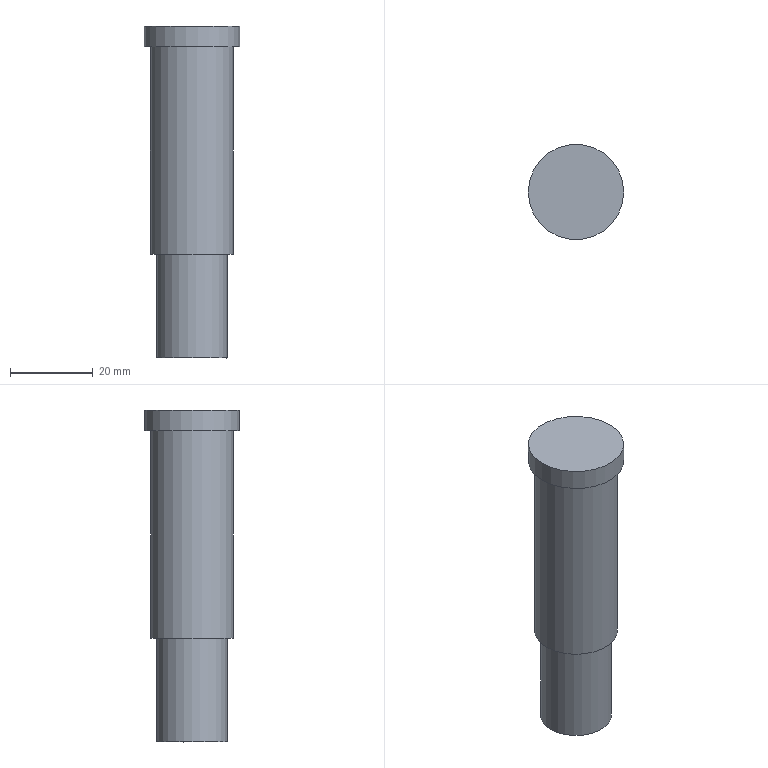Part | NX | features solid 2 | 1 solid | 7 faces | box 23 x 23 x 80 mm | volume 23527 mm3 | plane 4 | cylinder 3 | commonest cylinder face diameters 17.1 x1 20 x1 23 x1
STEP:
#1=CARTESIAN_POINT('',(471.302,165.949,8.192));
#2=VERTEX_POINT('',#1);
#3=CARTESIAN_POINT('',(461.302,165.949,8.192));
#4=DIRECTION('',(-0.000000502,-0.000000149,-1.));
#5=DIRECTION('',(1.,-0.000001668,-0.000000502));
#6=AXIS2_PLACEMENT_3D('',#3,#4,#5);
#7=CIRCLE('',#6,10.);
#8=EDGE_CURVE('',#2,#2,#7,.T.);
#9=ORIENTED_EDGE('',*,*,#8,.F.);
#10=EDGE_LOOP('',(#9));
#11=FACE_BOUND('',#10,.T.);
#12=CARTESIAN_POINT('',(471.302,165.949,58.192));
#13=VERTEX_POINT('',#12);
#14=CARTESIAN_POINT('',(461.302,165.949,58.192));
#15=DIRECTION('',(-0.000000502,-0.000000149,-1.));
#16=DIRECTION('',(1.,-0.000001668,-0.000000502));
#17=AXIS2_PLACEMENT_3D('',#14,#15,#16);
#18=CIRCLE('',#17,10.);
#19=EDGE_CURVE('',#13,#13,#18,.T.);
#20=ORIENTED_EDGE('',*,*,#19,.T.);
#21=EDGE_LOOP('',(#20));
#22=FACE_BOUND('',#21,.T.);
#23=CARTESIAN_POINT('',(461.302,165.949,63.192));
#24=DIRECTION('',(-0.000000502,-0.000000149,-1.));
#25=DIRECTION('',(-1.,0.000001668,0.000000502));
#26=AXIS2_PLACEMENT_3D('',#23,#24,#25);
#27=CYLINDRICAL_SURFACE('',#26,10.);
#28=ADVANCED_FACE('',(#11,#22),#27,.T.);
#29=CARTESIAN_POINT('',(469.852,165.949,8.192));
#30=VERTEX_POINT('',#29);
#31=CARTESIAN_POINT('',(461.302,165.949,8.192));
#32=DIRECTION('',(-0.000000502,-0.000000149,-1.));
#33=DIRECTION('',(1.,-0.000001668,-0.000000502));
#34=AXIS2_PLACEMENT_3D('',#31,#32,#33);
#35=CIRCLE('',#34,8.55);
#36=EDGE_CURVE('',#30,#30,#35,.T.);
#37=ORIENTED_EDGE('',*,*,#36,.F.);
#38=EDGE_LOOP('',(#37));
#39=FACE_BOUND('',#38,.T.);
#40=ORIENTED_EDGE('',*,*,#8,.T.);
#41=EDGE_LOOP('',(#40));
#42=FACE_BOUND('',#41,.T.);
#43=CARTESIAN_POINT('',(461.302,165.949,8.192));
#44=DIRECTION('',(0.000000502,0.000000149,1.));
#45=DIRECTION('',(1.,-0.000001668,-0.000000502));
#46=AXIS2_PLACEMENT_3D('',#43,#44,#45);
#47=PLANE('',#46);
#48=ADVANCED_FACE('',(#39,#42),#47,.F.);
#49=CARTESIAN_POINT('',(472.802,165.949,58.192));
#50=VERTEX_POINT('',#49);
#51=CARTESIAN_POINT('',(461.302,165.949,58.192));
#52=DIRECTION('',(-0.000000502,-0.000000149,-1.));
#53=DIRECTION('',(1.,-0.000001668,-0.000000502));
#54=AXIS2_PLACEMENT_3D('',#51,#52,#53);
#55=CIRCLE('',#54,11.5);
#56=EDGE_CURVE('',#50,#50,#55,.T.);
#57=ORIENTED_EDGE('',*,*,#56,.T.);
#58=EDGE_LOOP('',(#57));
#59=FACE_BOUND('',#58,.T.);
#60=ORIENTED_EDGE('',*,*,#19,.F.);
#61=EDGE_LOOP('',(#60));
#62=FACE_BOUND('',#61,.T.);
#63=CARTESIAN_POINT('',(461.302,165.949,58.192));
#64=DIRECTION('',(0.000000502,0.000000149,1.));
#65=DIRECTION('',(1.,-0.000001668,-0.000000502));
#66=AXIS2_PLACEMENT_3D('',#63,#64,#65);
#67=PLANE('',#66);
#68=ADVANCED_FACE('',(#59,#62),#67,.F.);
#69=ORIENTED_EDGE('',*,*,#56,.F.);
#70=EDGE_LOOP('',(#69));
#71=FACE_BOUND('',#70,.T.);
#72=CARTESIAN_POINT('',(472.802,165.949,63.192));
#73=VERTEX_POINT('',#72);
#74=CARTESIAN_POINT('',(461.302,165.949,63.192));
#75=DIRECTION('',(-0.000000502,-0.000000149,-1.));
#76=DIRECTION('',(1.,-0.000001668,-0.000000502));
#77=AXIS2_PLACEMENT_3D('',#74,#75,#76);
#78=CIRCLE('',#77,11.5);
#79=EDGE_CURVE('',#73,#73,#78,.T.);
#80=ORIENTED_EDGE('',*,*,#79,.T.);
#81=EDGE_LOOP('',(#80));
#82=FACE_BOUND('',#81,.T.);
#83=CARTESIAN_POINT('',(461.302,165.949,58.192));
#84=DIRECTION('',(0.000000502,0.000000149,1.));
#85=DIRECTION('',(1.,-0.000001668,-0.000000502));
#86=AXIS2_PLACEMENT_3D('',#83,#84,#85);
#87=CYLINDRICAL_SURFACE('',#86,11.5);
#88=ADVANCED_FACE('',(#71,#82),#87,.T.);
#89=ORIENTED_EDGE('',*,*,#79,.F.);
#90=EDGE_LOOP('',(#89));
#91=FACE_BOUND('',#90,.T.);
#92=CARTESIAN_POINT('',(461.302,165.949,63.192));
#93=DIRECTION('',(0.000000502,0.000000149,1.));
#94=DIRECTION('',(1.,-0.000001668,-0.000000502));
#95=AXIS2_PLACEMENT_3D('',#92,#93,#94);
#96=PLANE('',#95);
#97=ADVANCED_FACE('',(#91),#96,.T.);
#98=CARTESIAN_POINT('',(469.852,165.949,-16.808));
#99=VERTEX_POINT('',#98);
#100=CARTESIAN_POINT('',(461.302,165.949,-16.808));
#101=DIRECTION('',(-0.000000502,-0.000000149,-1.));
#102=DIRECTION('',(1.,-0.000001668,-0.000000502));
#103=AXIS2_PLACEMENT_3D('',#100,#101,#102);
#104=CIRCLE('',#103,8.55);
#105=EDGE_CURVE('',#99,#99,#104,.T.);
#106=ORIENTED_EDGE('',*,*,#105,.F.);
#107=EDGE_LOOP('',(#106));
#108=FACE_BOUND('',#107,.T.);
#109=ORIENTED_EDGE('',*,*,#36,.T.);
#110=EDGE_LOOP('',(#109));
#111=FACE_BOUND('',#110,.T.);
#112=CARTESIAN_POINT('',(461.302,165.949,-16.808));
#113=DIRECTION('',(0.000000502,0.000000149,1.));
#114=DIRECTION('',(1.,-0.000001668,-0.000000502));
#115=AXIS2_PLACEMENT_3D('',#112,#113,#114);
#116=CYLINDRICAL_SURFACE('',#115,8.55);
#117=ADVANCED_FACE('',(#108,#111),#116,.T.);
#118=ORIENTED_EDGE('',*,*,#105,.T.);
#119=EDGE_LOOP('',(#118));
#120=FACE_BOUND('',#119,.T.);
#121=CARTESIAN_POINT('',(461.302,165.949,-16.808));
#122=DIRECTION('',(0.000000502,0.000000149,1.));
#123=DIRECTION('',(1.,-0.000001668,-0.000000502));
#124=AXIS2_PLACEMENT_3D('',#121,#122,#123);
#125=PLANE('',#124);
#126=ADVANCED_FACE('',(#120),#125,.F.);
#127=CLOSED_SHELL('',(#28,#48,#68,#88,#97,#117,#126));
#128=MANIFOLD_SOLID_BREP('',#127);
#129=(LENGTH_UNIT()NAMED_UNIT(*)SI_UNIT(.MILLI.,.METRE.));
#130=UNCERTAINTY_MEASURE_WITH_UNIT(LENGTH_MEASURE(0.00001),#129,'','');
#131=(NAMED_UNIT(*)PLANE_ANGLE_UNIT()SI_UNIT($,.RADIAN.));
#132=(NAMED_UNIT(*)SI_UNIT($,.STERADIAN.)SOLID_ANGLE_UNIT());
#133=(GEOMETRIC_REPRESENTATION_CONTEXT(3)GLOBAL_UNCERTAINTY_ASSIGNED_CONTEXT((#130))GLOBAL_UNIT_ASSIGNED_CONTEXT((#129,#131,#132))REPRESENTATION_CONTEXT('',''));
#134=ADVANCED_BREP_SHAPE_REPRESENTATION('',(#128),#133);